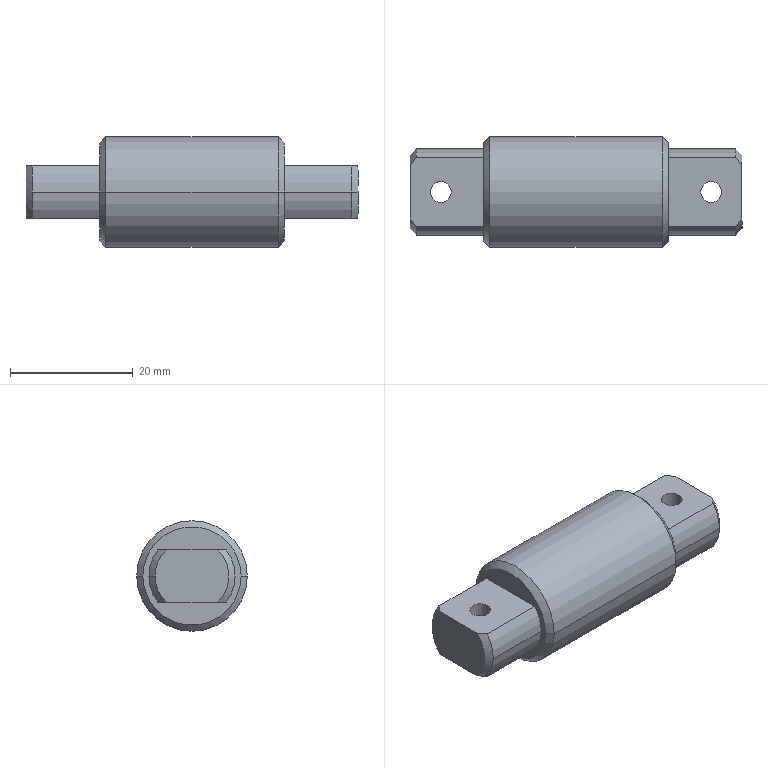Part | STEP file | Chain connecting rod | 1 solid | 30 faces | box 54 x 18 x 18 mm | volume 10076 mm3 | cylinder 12 | cone 10 | plane 8 | commonest cylinder face diameters 14 x6 3.4 x4 18 x2